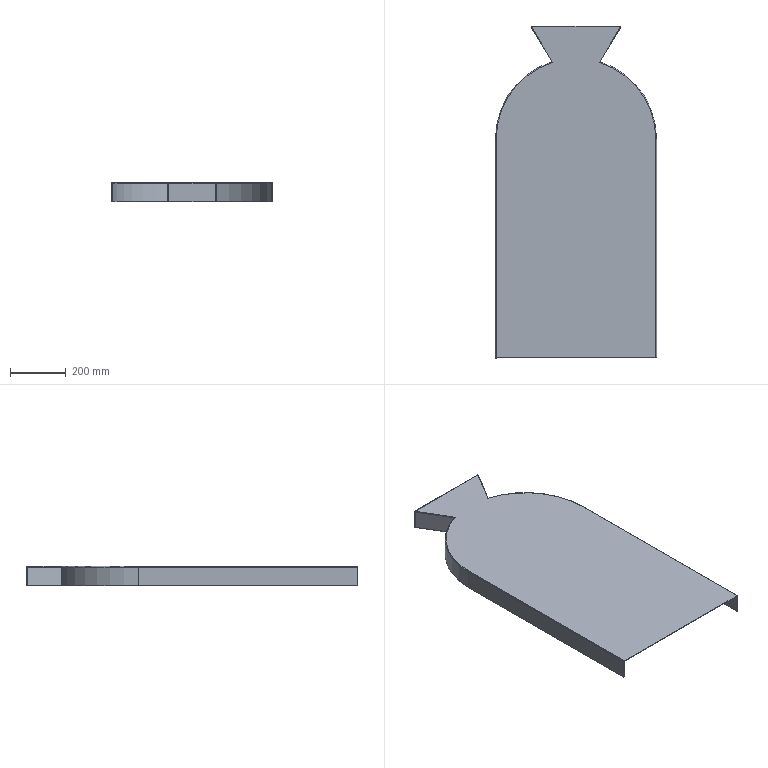Part | SolidWorks | features EdgeFlange 5, 3DProfileFeature 2, FlatPattern 1, ICE 1, SMBaseFlange 1, SheetMetal 1 | 1 solid | 62 faces | box 578 x 1192 x 70 mm | volume 1625565 mm3 | plane 42 | cylinder 14 | torus 4 | spline 2 | commonest cylinder face diameters 1.473 x5 5.473 x5 574 x2 578 x2